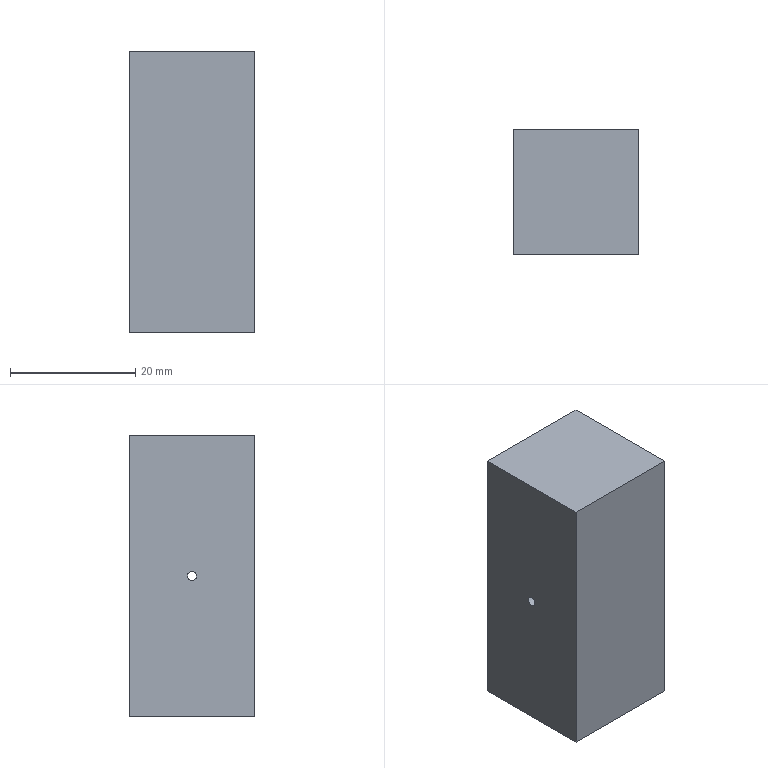Part | STEP file | SN10_016_001-02_BLOCO | 1 solid | 8 faces | box 20 x 20 x 45 mm | volume 16964 mm3 | plane 6 | cylinder 1 | cone 1 | commonest cylinder face diameters 8.376 x1
STEP:
#1=CARTESIAN_POINT('',(0.,0.,0.));
#2=DIRECTION('',(0.,0.,1.));
#3=DIRECTION('',(1.,0.,0.));
#4=AXIS2_PLACEMENT_3D('',#1,#2,#3);
#5=CARTESIAN_POINT('',(5341.,-1241.325,70.492));
#6=VERTEX_POINT('',#5);
#7=CARTESIAN_POINT('',(5341.,-1245.,72.5));
#8=DIRECTION('',(-1.,0.,0.));
#9=DIRECTION('',(0.,1.,0.));
#10=AXIS2_PLACEMENT_3D('',#7,#8,#9);
#11=CIRCLE('',#10,4.188);
#12=CARTESIAN_POINT('',(5340.9,-1245.,72.5));
#13=DIRECTION('',(-1.,0.,0.));
#14=DIRECTION('',(0.,0.8776,-0.4794));
#15=AXIS2_PLACEMENT_3D('',#12,#13,#14);
#16=CYLINDRICAL_SURFACE('',#15,4.188);
#17=CARTESIAN_POINT('',(-0.5,-0.1));
#18=DIRECTION('',(1.,0.));
#19=VECTOR('',#18,1.);
#20=LINE('',#17,#19);
#21=(GEOMETRIC_REPRESENTATION_CONTEXT(2)PARAMETRIC_REPRESENTATION_CONTEXT()REPRESENTATION_CONTEXT('',''));
#22=DEFINITIONAL_REPRESENTATION('',(#20),#21);
#23=PCURVE('',#16,#22);
#24=CARTESIAN_POINT('',(5341.,0.,0.));
#25=DIRECTION('',(1.,0.,0.));
#26=DIRECTION('',(0.,0.,-1.));
#27=AXIS2_PLACEMENT_3D('',#24,#25,#26);
#28=PLANE('',#27);
#29=CARTESIAN_POINT('',(-72.5,-1240.812));
#30=CARTESIAN_POINT('',(-65.246,-1240.812));
#31=CARTESIAN_POINT('',(-68.873,-1247.094));
#32=CARTESIAN_POINT('',(-72.5,-1253.376));
#33=CARTESIAN_POINT('',(-76.127,-1247.094));
#34=CARTESIAN_POINT('',(-79.754,-1240.812));
#35=CARTESIAN_POINT('',(-72.5,-1240.812));
#36=(BOUNDED_CURVE()B_SPLINE_CURVE(2,(#29,#30,#31,#32,#33,#34,#35),.UNSPECIFIED.,.T.,.F.)B_SPLINE_CURVE_WITH_KNOTS((1,2,2,2,2,1),(-2.094,0.,2.094,4.189,6.283,8.378),.UNSPECIFIED.)CURVE()GEOMETRIC_REPRESENTATION_ITEM()RATIONAL_B_SPLINE_CURVE((1.,0.5,1.,0.5,1.,0.5,1.))REPRESENTATION_ITEM(''));
#37=(GEOMETRIC_REPRESENTATION_CONTEXT(2)PARAMETRIC_REPRESENTATION_CONTEXT()REPRESENTATION_CONTEXT('',''));
#38=DEFINITIONAL_REPRESENTATION('',(#36),#37);
#39=PCURVE('',#28,#38);
#40=SURFACE_CURVE('',#11,(#23,#39),.PCURVE_S1.);
#41=EDGE_CURVE('',#6,#6,#40,.T.);
#42=ORIENTED_EDGE('',*,*,#41,.T.);
#43=CARTESIAN_POINT('',(5323.,-1241.325,70.492));
#44=VERTEX_POINT('',#43);
#45=CARTESIAN_POINT('',(5341.,-1241.325,70.492));
#46=CARTESIAN_POINT('',(5323.,-1241.325,70.492));
#47=B_SPLINE_CURVE_WITH_KNOTS('',1,(#45,#46),.UNSPECIFIED.,.F.,.F.,(2,2),(-0.1,17.9),.PIECEWISE_BEZIER_KNOTS.);
#48=CARTESIAN_POINT('',(6.283,0.));
#49=DIRECTION('',(0.,1.));
#50=VECTOR('',#49,1.);
#51=LINE('',#48,#50);
#52=(GEOMETRIC_REPRESENTATION_CONTEXT(2)PARAMETRIC_REPRESENTATION_CONTEXT()REPRESENTATION_CONTEXT('',''));
#53=DEFINITIONAL_REPRESENTATION('',(#51),#52);
#54=PCURVE('',#16,#53);
#55=CARTESIAN_POINT('',(0.,0.));
#56=DIRECTION('',(0.,1.));
#57=VECTOR('',#56,1.);
#58=LINE('',#55,#57);
#59=(GEOMETRIC_REPRESENTATION_CONTEXT(2)PARAMETRIC_REPRESENTATION_CONTEXT()REPRESENTATION_CONTEXT('',''));
#60=DEFINITIONAL_REPRESENTATION('',(#58),#59);
#61=PCURVE('',#16,#60);
#62=SEAM_CURVE('',#47,(#54,#61),.PCURVE_S1.);
#63=EDGE_CURVE('',#6,#44,#62,.T.);
#64=ORIENTED_EDGE('',*,*,#63,.T.);
#65=CARTESIAN_POINT('',(5323.,-1245.,72.5));
#66=DIRECTION('',(-1.,0.,0.));
#67=DIRECTION('',(0.,1.,0.));
#68=AXIS2_PLACEMENT_3D('',#65,#66,#67);
#69=CIRCLE('',#68,4.188);
#70=CARTESIAN_POINT('',(-0.5,17.9));
#71=DIRECTION('',(1.,0.));
#72=VECTOR('',#71,1.);
#73=LINE('',#70,#72);
#74=(GEOMETRIC_REPRESENTATION_CONTEXT(2)PARAMETRIC_REPRESENTATION_CONTEXT()REPRESENTATION_CONTEXT('',''));
#75=DEFINITIONAL_REPRESENTATION('',(#73),#74);
#76=PCURVE('',#16,#75);
#77=CARTESIAN_POINT('',(5321.159,-1245.,72.5));
#78=DIRECTION('',(1.,0.,0.));
#79=DIRECTION('',(0.,0.8776,-0.4794));
#80=AXIS2_PLACEMENT_3D('',#77,#78,#79);
#81=CONICAL_SURFACE('',#80,1.,1.047);
#82=CARTESIAN_POINT('',(6.783,1.841));
#83=DIRECTION('',(-1.,0.));
#84=VECTOR('',#83,1.);
#85=LINE('',#82,#84);
#86=(GEOMETRIC_REPRESENTATION_CONTEXT(2)PARAMETRIC_REPRESENTATION_CONTEXT()REPRESENTATION_CONTEXT('',''));
#87=DEFINITIONAL_REPRESENTATION('',(#85),#86);
#88=PCURVE('',#81,#87);
#89=SURFACE_CURVE('',#69,(#76,#88),.PCURVE_S1.);
#90=EDGE_CURVE('',#44,#44,#89,.T.);
#91=ORIENTED_EDGE('',*,*,#90,.F.);
#92=ORIENTED_EDGE('',*,*,#63,.F.);
#93=EDGE_LOOP('',(#42,#64,#91,#92));
#94=FACE_BOUND('',#93,.F.);
#95=ADVANCED_FACE('',(#94),#16,.F.);
#96=CARTESIAN_POINT('',(5321.,-1245.635,72.847));
#97=VERTEX_POINT('',#96);
#98=CARTESIAN_POINT('',(5321.,-1244.365,72.153));
#99=VERTEX_POINT('',#98);
#100=CARTESIAN_POINT('',(5321.,-1245.,72.5));
#101=DIRECTION('',(1.,0.,0.));
#102=DIRECTION('',(0.,1.,0.));
#103=AXIS2_PLACEMENT_3D('',#100,#101,#102);
#104=CIRCLE('',#103,0.7239);
#105=CARTESIAN_POINT('',(0.5,-0.1594));
#106=DIRECTION('',(1.,0.));
#107=VECTOR('',#106,1.);
#108=LINE('',#105,#107);
#109=(GEOMETRIC_REPRESENTATION_CONTEXT(2)PARAMETRIC_REPRESENTATION_CONTEXT()REPRESENTATION_CONTEXT('',''));
#110=DEFINITIONAL_REPRESENTATION('',(#108),#109);
#111=PCURVE('',#81,#110);
#112=CARTESIAN_POINT('',(5321.,0.,0.));
#113=DIRECTION('',(1.,0.,0.));
#114=DIRECTION('',(0.,0.,-1.));
#115=AXIS2_PLACEMENT_3D('',#112,#113,#114);
#116=PLANE('',#115);
#117=CARTESIAN_POINT('',(-72.5,-1245.));
#118=DIRECTION('',(0.,1.));
#119=AXIS2_PLACEMENT_2D('',#117,#118);
#120=CIRCLE('',#119,0.7239);
#121=(GEOMETRIC_REPRESENTATION_CONTEXT(2)PARAMETRIC_REPRESENTATION_CONTEXT()REPRESENTATION_CONTEXT('',''));
#122=DEFINITIONAL_REPRESENTATION('',(#120),#121);
#123=PCURVE('',#116,#122);
#124=SURFACE_CURVE('',#104,(#111,#123),.PCURVE_S1.);
#125=EDGE_CURVE('',#97,#99,#124,.T.);
#126=ORIENTED_EDGE('',*,*,#125,.T.);
#127=CARTESIAN_POINT('',(5321.,-1244.365,72.153));
#128=CARTESIAN_POINT('',(5323.,-1241.325,70.492));
#129=B_SPLINE_CURVE_WITH_KNOTS('',1,(#127,#128),.UNSPECIFIED.,.F.,.F.,(2,2),(-0.3188,3.681),.PIECEWISE_BEZIER_KNOTS.);
#130=CARTESIAN_POINT('',(6.283,0.));
#131=DIRECTION('',(0.,1.));
#132=VECTOR('',#131,1.);
#133=LINE('',#130,#132);
#134=(GEOMETRIC_REPRESENTATION_CONTEXT(2)PARAMETRIC_REPRESENTATION_CONTEXT()REPRESENTATION_CONTEXT('',''));
#135=DEFINITIONAL_REPRESENTATION('',(#133),#134);
#136=PCURVE('',#81,#135);
#137=CARTESIAN_POINT('',(0.,0.));
#138=DIRECTION('',(0.,1.));
#139=VECTOR('',#138,1.);
#140=LINE('',#137,#139);
#141=(GEOMETRIC_REPRESENTATION_CONTEXT(2)PARAMETRIC_REPRESENTATION_CONTEXT()REPRESENTATION_CONTEXT('',''));
#142=DEFINITIONAL_REPRESENTATION('',(#140),#141);
#143=PCURVE('',#81,#142);
#144=SEAM_CURVE('',#129,(#136,#143),.PCURVE_S1.);
#145=EDGE_CURVE('',#99,#44,#144,.T.);
#146=ORIENTED_EDGE('',*,*,#145,.T.);
#147=ORIENTED_EDGE('',*,*,#90,.T.);
#148=ORIENTED_EDGE('',*,*,#145,.F.);
#149=CARTESIAN_POINT('',(5321.,-1245.,72.5));
#150=DIRECTION('',(1.,0.,0.));
#151=DIRECTION('',(0.,1.,0.));
#152=AXIS2_PLACEMENT_3D('',#149,#150,#151);
#153=CIRCLE('',#152,0.7239);
#154=CARTESIAN_POINT('',(-5.783,-0.1594));
#155=DIRECTION('',(1.,0.));
#156=VECTOR('',#155,1.);
#157=LINE('',#154,#156);
#158=(GEOMETRIC_REPRESENTATION_CONTEXT(2)PARAMETRIC_REPRESENTATION_CONTEXT()REPRESENTATION_CONTEXT('',''));
#159=DEFINITIONAL_REPRESENTATION('',(#157),#158);
#160=PCURVE('',#81,#159);
#161=CARTESIAN_POINT('',(-72.5,-1245.));
#162=DIRECTION('',(0.,1.));
#163=AXIS2_PLACEMENT_2D('',#161,#162);
#164=CIRCLE('',#163,0.7239);
#165=(GEOMETRIC_REPRESENTATION_CONTEXT(2)PARAMETRIC_REPRESENTATION_CONTEXT()REPRESENTATION_CONTEXT('',''));
#166=DEFINITIONAL_REPRESENTATION('',(#164),#165);
#167=PCURVE('',#116,#166);
#168=SURFACE_CURVE('',#153,(#160,#167),.PCURVE_S1.);
#169=EDGE_CURVE('',#99,#97,#168,.T.);
#170=ORIENTED_EDGE('',*,*,#169,.T.);
#171=EDGE_LOOP('',(#126,#146,#147,#148,#170));
#172=FACE_BOUND('',#171,.F.);
#173=ADVANCED_FACE('',(#172),#81,.F.);
#174=CARTESIAN_POINT('',(5341.,-1255.,95.));
#175=VERTEX_POINT('',#174);
#176=CARTESIAN_POINT('',(5341.,-1255.,50.));
#177=VERTEX_POINT('',#176);
#178=CARTESIAN_POINT('',(5341.,-1255.,95.));
#179=DIRECTION('',(0.,0.,-1.));
#180=VECTOR('',#179,1.);
#181=LINE('',#178,#180);
#182=CARTESIAN_POINT('',(-95.,-1255.));
#183=DIRECTION('',(1.,0.));
#184=VECTOR('',#183,1.);
#185=LINE('',#182,#184);
#186=(GEOMETRIC_REPRESENTATION_CONTEXT(2)PARAMETRIC_REPRESENTATION_CONTEXT()REPRESENTATION_CONTEXT('',''));
#187=DEFINITIONAL_REPRESENTATION('',(#185),#186);
#188=PCURVE('',#28,#187);
#189=CARTESIAN_POINT('',(5321.,-1255.,95.));
#190=DIRECTION('',(0.,-1.,0.));
#191=DIRECTION('',(0.,0.,-1.));
#192=AXIS2_PLACEMENT_3D('',#189,#190,#191);
#193=PLANE('',#192);
#194=CARTESIAN_POINT('',(0.,20.));
#195=DIRECTION('',(1.,0.));
#196=VECTOR('',#195,1.);
#197=LINE('',#194,#196);
#198=(GEOMETRIC_REPRESENTATION_CONTEXT(2)PARAMETRIC_REPRESENTATION_CONTEXT()REPRESENTATION_CONTEXT('',''));
#199=DEFINITIONAL_REPRESENTATION('',(#197),#198);
#200=PCURVE('',#193,#199);
#201=SURFACE_CURVE('',#181,(#188,#200),.PCURVE_S1.);
#202=EDGE_CURVE('',#175,#177,#201,.T.);
#203=ORIENTED_EDGE('',*,*,#202,.T.);
#204=CARTESIAN_POINT('',(5341.,-1235.,50.));
#205=VERTEX_POINT('',#204);
#206=CARTESIAN_POINT('',(5341.,-1235.,50.));
#207=DIRECTION('',(0.,-1.,0.));
#208=VECTOR('',#207,1.);
#209=LINE('',#206,#208);
#210=CARTESIAN_POINT('',(-50.,-1235.));
#211=DIRECTION('',(0.,-1.));
#212=VECTOR('',#211,1.);
#213=LINE('',#210,#212);
#214=(GEOMETRIC_REPRESENTATION_CONTEXT(2)PARAMETRIC_REPRESENTATION_CONTEXT()REPRESENTATION_CONTEXT('',''));
#215=DEFINITIONAL_REPRESENTATION('',(#213),#214);
#216=PCURVE('',#28,#215);
#217=CARTESIAN_POINT('',(5321.,-1235.,50.));
#218=DIRECTION('',(0.,0.,1.));
#219=DIRECTION('',(1.,0.,0.));
#220=AXIS2_PLACEMENT_3D('',#217,#218,#219);
#221=PLANE('',#220);
#222=CARTESIAN_POINT('',(20.,0.));
#223=DIRECTION('',(0.,-1.));
#224=VECTOR('',#223,1.);
#225=LINE('',#222,#224);
#226=(GEOMETRIC_REPRESENTATION_CONTEXT(2)PARAMETRIC_REPRESENTATION_CONTEXT()REPRESENTATION_CONTEXT('',''));
#227=DEFINITIONAL_REPRESENTATION('',(#225),#226);
#228=PCURVE('',#221,#227);
#229=SURFACE_CURVE('',#209,(#216,#228),.PCURVE_S1.);
#230=EDGE_CURVE('',#205,#177,#229,.T.);
#231=ORIENTED_EDGE('',*,*,#230,.F.);
#232=CARTESIAN_POINT('',(5341.,-1235.,95.));
#233=VERTEX_POINT('',#232);
#234=CARTESIAN_POINT('',(5341.,-1235.,50.));
#235=DIRECTION('',(0.,0.,1.));
#236=VECTOR('',#235,1.);
#237=LINE('',#234,#236);
#238=CARTESIAN_POINT('',(-50.,-1235.));
#239=DIRECTION('',(-1.,0.));
#240=VECTOR('',#239,1.);
#241=LINE('',#238,#240);
#242=(GEOMETRIC_REPRESENTATION_CONTEXT(2)PARAMETRIC_REPRESENTATION_CONTEXT()REPRESENTATION_CONTEXT('',''));
#243=DEFINITIONAL_REPRESENTATION('',(#241),#242);
#244=PCURVE('',#28,#243);
#245=CARTESIAN_POINT('',(5321.,-1235.,50.));
#246=DIRECTION('',(0.,1.,0.));
#247=DIRECTION('',(0.,0.,1.));
#248=AXIS2_PLACEMENT_3D('',#245,#246,#247);
#249=PLANE('',#248);
#250=CARTESIAN_POINT('',(0.,20.));
#251=DIRECTION('',(1.,0.));
#252=VECTOR('',#251,1.);
#253=LINE('',#250,#252);
#254=(GEOMETRIC_REPRESENTATION_CONTEXT(2)PARAMETRIC_REPRESENTATION_CONTEXT()REPRESENTATION_CONTEXT('',''));
#255=DEFINITIONAL_REPRESENTATION('',(#253),#254);
#256=PCURVE('',#249,#255);
#257=SURFACE_CURVE('',#237,(#244,#256),.PCURVE_S1.);
#258=EDGE_CURVE('',#205,#233,#257,.T.);
#259=ORIENTED_EDGE('',*,*,#258,.T.);
#260=CARTESIAN_POINT('',(5341.,-1255.,95.));
#261=DIRECTION('',(0.,1.,0.));
#262=VECTOR('',#261,1.);
#263=LINE('',#260,#262);
#264=CARTESIAN_POINT('',(-95.,-1255.));
#265=DIRECTION('',(0.,1.));
#266=VECTOR('',#265,1.);
#267=LINE('',#264,#266);
#268=(GEOMETRIC_REPRESENTATION_CONTEXT(2)PARAMETRIC_REPRESENTATION_CONTEXT()REPRESENTATION_CONTEXT('',''));
#269=DEFINITIONAL_REPRESENTATION('',(#267),#268);
#270=PCURVE('',#28,#269);
#271=CARTESIAN_POINT('',(5321.,-1255.,95.));
#272=DIRECTION('',(0.,0.,-1.));
#273=DIRECTION('',(-1.,0.,0.));
#274=AXIS2_PLACEMENT_3D('',#271,#272,#273);
#275=PLANE('',#274);
#276=CARTESIAN_POINT('',(-20.,0.));
#277=DIRECTION('',(0.,1.));
#278=VECTOR('',#277,1.);
#279=LINE('',#276,#278);
#280=(GEOMETRIC_REPRESENTATION_CONTEXT(2)PARAMETRIC_REPRESENTATION_CONTEXT()REPRESENTATION_CONTEXT('',''));
#281=DEFINITIONAL_REPRESENTATION('',(#279),#280);
#282=PCURVE('',#275,#281);
#283=SURFACE_CURVE('',#263,(#270,#282),.PCURVE_S1.);
#284=EDGE_CURVE('',#175,#233,#283,.T.);
#285=ORIENTED_EDGE('',*,*,#284,.F.);
#286=EDGE_LOOP('',(#203,#231,#259,#285));
#287=FACE_BOUND('',#286,.T.);
#288=ORIENTED_EDGE('',*,*,#41,.T.);
#289=EDGE_LOOP('',(#288));
#290=FACE_BOUND('',#289,.T.);
#291=ADVANCED_FACE('',(#287,#290),#28,.T.);
#292=CARTESIAN_POINT('',(5321.,-1255.,95.));
#293=VERTEX_POINT('',#292);
#294=CARTESIAN_POINT('',(5321.,-1255.,95.));
#295=DIRECTION('',(1.,0.,0.));
#296=VECTOR('',#295,1.);
#297=LINE('',#294,#296);
#298=CARTESIAN_POINT('',(0.,0.));
#299=DIRECTION('',(0.,1.));
#300=VECTOR('',#299,1.);
#301=LINE('',#298,#300);
#302=(GEOMETRIC_REPRESENTATION_CONTEXT(2)PARAMETRIC_REPRESENTATION_CONTEXT()REPRESENTATION_CONTEXT('',''));
#303=DEFINITIONAL_REPRESENTATION('',(#301),#302);
#304=PCURVE('',#193,#303);
#305=CARTESIAN_POINT('',(0.,0.));
#306=DIRECTION('',(-1.,0.));
#307=VECTOR('',#306,1.);
#308=LINE('',#305,#307);
#309=(GEOMETRIC_REPRESENTATION_CONTEXT(2)PARAMETRIC_REPRESENTATION_CONTEXT()REPRESENTATION_CONTEXT('',''));
#310=DEFINITIONAL_REPRESENTATION('',(#308),#309);
#311=PCURVE('',#275,#310);
#312=SURFACE_CURVE('',#297,(#304,#311),.PCURVE_S1.);
#313=EDGE_CURVE('',#293,#175,#312,.T.);
#314=ORIENTED_EDGE('',*,*,#313,.F.);
#315=CARTESIAN_POINT('',(5321.,-1255.,50.));
#316=VERTEX_POINT('',#315);
#317=CARTESIAN_POINT('',(5321.,-1255.,95.));
#318=DIRECTION('',(0.,0.,-1.));
#319=VECTOR('',#318,1.);
#320=LINE('',#317,#319);
#321=CARTESIAN_POINT('',(0.,0.));
#322=DIRECTION('',(1.,0.));
#323=VECTOR('',#322,1.);
#324=LINE('',#321,#323);
#325=(GEOMETRIC_REPRESENTATION_CONTEXT(2)PARAMETRIC_REPRESENTATION_CONTEXT()REPRESENTATION_CONTEXT('',''));
#326=DEFINITIONAL_REPRESENTATION('',(#324),#325);
#327=PCURVE('',#193,#326);
#328=CARTESIAN_POINT('',(-95.,-1255.));
#329=DIRECTION('',(1.,0.));
#330=VECTOR('',#329,1.);
#331=LINE('',#328,#330);
#332=(GEOMETRIC_REPRESENTATION_CONTEXT(2)PARAMETRIC_REPRESENTATION_CONTEXT()REPRESENTATION_CONTEXT('',''));
#333=DEFINITIONAL_REPRESENTATION('',(#331),#332);
#334=PCURVE('',#116,#333);
#335=SURFACE_CURVE('',#320,(#327,#334),.PCURVE_S1.);
#336=EDGE_CURVE('',#293,#316,#335,.T.);
#337=ORIENTED_EDGE('',*,*,#336,.T.);
#338=CARTESIAN_POINT('',(5321.,-1255.,50.));
#339=DIRECTION('',(1.,0.,0.));
#340=VECTOR('',#339,1.);
#341=LINE('',#338,#340);
#342=CARTESIAN_POINT('',(45.,0.));
#343=DIRECTION('',(0.,1.));
#344=VECTOR('',#343,1.);
#345=LINE('',#342,#344);
#346=(GEOMETRIC_REPRESENTATION_CONTEXT(2)PARAMETRIC_REPRESENTATION_CONTEXT()REPRESENTATION_CONTEXT('',''));
#347=DEFINITIONAL_REPRESENTATION('',(#345),#346);
#348=PCURVE('',#193,#347);
#349=CARTESIAN_POINT('',(0.,-20.));
#350=DIRECTION('',(1.,0.));
#351=VECTOR('',#350,1.);
#352=LINE('',#349,#351);
#353=(GEOMETRIC_REPRESENTATION_CONTEXT(2)PARAMETRIC_REPRESENTATION_CONTEXT()REPRESENTATION_CONTEXT('',''));
#354=DEFINITIONAL_REPRESENTATION('',(#352),#353);
#355=PCURVE('',#221,#354);
#356=SURFACE_CURVE('',#341,(#348,#355),.PCURVE_S1.);
#357=EDGE_CURVE('',#316,#177,#356,.T.);
#358=ORIENTED_EDGE('',*,*,#357,.T.);
#359=ORIENTED_EDGE('',*,*,#202,.F.);
#360=EDGE_LOOP('',(#314,#337,#358,#359));
#361=FACE_BOUND('',#360,.T.);
#362=ADVANCED_FACE('',(#361),#193,.T.);
#363=ORIENTED_EDGE('',*,*,#357,.F.);
#364=CARTESIAN_POINT('',(5321.,-1235.,50.));
#365=VERTEX_POINT('',#364);
#366=CARTESIAN_POINT('',(5321.,-1235.,50.));
#367=DIRECTION('',(0.,-1.,0.));
#368=VECTOR('',#367,1.);
#369=LINE('',#366,#368);
#370=CARTESIAN_POINT('',(0.,0.));
#371=DIRECTION('',(0.,-1.));
#372=VECTOR('',#371,1.);
#373=LINE('',#370,#372);
#374=(GEOMETRIC_REPRESENTATION_CONTEXT(2)PARAMETRIC_REPRESENTATION_CONTEXT()REPRESENTATION_CONTEXT('',''));
#375=DEFINITIONAL_REPRESENTATION('',(#373),#374);
#376=PCURVE('',#221,#375);
#377=CARTESIAN_POINT('',(-50.,-1235.));
#378=DIRECTION('',(0.,-1.));
#379=VECTOR('',#378,1.);
#380=LINE('',#377,#379);
#381=(GEOMETRIC_REPRESENTATION_CONTEXT(2)PARAMETRIC_REPRESENTATION_CONTEXT()REPRESENTATION_CONTEXT('',''));
#382=DEFINITIONAL_REPRESENTATION('',(#380),#381);
#383=PCURVE('',#116,#382);
#384=SURFACE_CURVE('',#369,(#376,#383),.PCURVE_S1.);
#385=EDGE_CURVE('',#365,#316,#384,.T.);
#386=ORIENTED_EDGE('',*,*,#385,.F.);
#387=CARTESIAN_POINT('',(5321.,-1235.,50.));
#388=DIRECTION('',(1.,0.,0.));
#389=VECTOR('',#388,1.);
#390=LINE('',#387,#389);
#391=CARTESIAN_POINT('',(0.,0.));
#392=DIRECTION('',(1.,0.));
#393=VECTOR('',#392,1.);
#394=LINE('',#391,#393);
#395=(GEOMETRIC_REPRESENTATION_CONTEXT(2)PARAMETRIC_REPRESENTATION_CONTEXT()REPRESENTATION_CONTEXT('',''));
#396=DEFINITIONAL_REPRESENTATION('',(#394),#395);
#397=PCURVE('',#221,#396);
#398=CARTESIAN_POINT('',(0.,0.));
#399=DIRECTION('',(0.,1.));
#400=VECTOR('',#399,1.);
#401=LINE('',#398,#400);
#402=(GEOMETRIC_REPRESENTATION_CONTEXT(2)PARAMETRIC_REPRESENTATION_CONTEXT()REPRESENTATION_CONTEXT('',''));
#403=DEFINITIONAL_REPRESENTATION('',(#401),#402);
#404=PCURVE('',#249,#403);
#405=SURFACE_CURVE('',#390,(#397,#404),.PCURVE_S1.);
#406=EDGE_CURVE('',#365,#205,#405,.T.);
#407=ORIENTED_EDGE('',*,*,#406,.T.);
#408=ORIENTED_EDGE('',*,*,#230,.T.);
#409=EDGE_LOOP('',(#363,#386,#407,#408));
#410=FACE_BOUND('',#409,.T.);
#411=ADVANCED_FACE('',(#410),#221,.F.);
#412=ORIENTED_EDGE('',*,*,#406,.F.);
#413=CARTESIAN_POINT('',(5321.,-1235.,95.));
#414=VERTEX_POINT('',#413);
#415=CARTESIAN_POINT('',(5321.,-1235.,50.));
#416=DIRECTION('',(0.,0.,1.));
#417=VECTOR('',#416,1.);
#418=LINE('',#415,#417);
#419=CARTESIAN_POINT('',(0.,0.));
#420=DIRECTION('',(1.,0.));
#421=VECTOR('',#420,1.);
#422=LINE('',#419,#421);
#423=(GEOMETRIC_REPRESENTATION_CONTEXT(2)PARAMETRIC_REPRESENTATION_CONTEXT()REPRESENTATION_CONTEXT('',''));
#424=DEFINITIONAL_REPRESENTATION('',(#422),#423);
#425=PCURVE('',#249,#424);
#426=CARTESIAN_POINT('',(-50.,-1235.));
#427=DIRECTION('',(-1.,0.));
#428=VECTOR('',#427,1.);
#429=LINE('',#426,#428);
#430=(GEOMETRIC_REPRESENTATION_CONTEXT(2)PARAMETRIC_REPRESENTATION_CONTEXT()REPRESENTATION_CONTEXT('',''));
#431=DEFINITIONAL_REPRESENTATION('',(#429),#430);
#432=PCURVE('',#116,#431);
#433=SURFACE_CURVE('',#418,(#425,#432),.PCURVE_S1.);
#434=EDGE_CURVE('',#365,#414,#433,.T.);
#435=ORIENTED_EDGE('',*,*,#434,.T.);
#436=CARTESIAN_POINT('',(5321.,-1235.,95.));
#437=DIRECTION('',(1.,0.,0.));
#438=VECTOR('',#437,1.);
#439=LINE('',#436,#438);
#440=CARTESIAN_POINT('',(45.,0.));
#441=DIRECTION('',(0.,1.));
#442=VECTOR('',#441,1.);
#443=LINE('',#440,#442);
#444=(GEOMETRIC_REPRESENTATION_CONTEXT(2)PARAMETRIC_REPRESENTATION_CONTEXT()REPRESENTATION_CONTEXT('',''));
#445=DEFINITIONAL_REPRESENTATION('',(#443),#444);
#446=PCURVE('',#249,#445);
#447=CARTESIAN_POINT('',(0.,20.));
#448=DIRECTION('',(-1.,0.));
#449=VECTOR('',#448,1.);
#450=LINE('',#447,#449);
#451=(GEOMETRIC_REPRESENTATION_CONTEXT(2)PARAMETRIC_REPRESENTATION_CONTEXT()REPRESENTATION_CONTEXT('',''));
#452=DEFINITIONAL_REPRESENTATION('',(#450),#451);
#453=PCURVE('',#275,#452);
#454=SURFACE_CURVE('',#439,(#446,#453),.PCURVE_S1.);
#455=EDGE_CURVE('',#414,#233,#454,.T.);
#456=ORIENTED_EDGE('',*,*,#455,.T.);
#457=ORIENTED_EDGE('',*,*,#258,.F.);
#458=EDGE_LOOP('',(#412,#435,#456,#457));
#459=FACE_BOUND('',#458,.T.);
#460=ADVANCED_FACE('',(#459),#249,.T.);
#461=ORIENTED_EDGE('',*,*,#455,.F.);
#462=CARTESIAN_POINT('',(5321.,-1255.,95.));
#463=DIRECTION('',(0.,1.,0.));
#464=VECTOR('',#463,1.);
#465=LINE('',#462,#464);
#466=CARTESIAN_POINT('',(0.,0.));
#467=DIRECTION('',(0.,1.));
#468=VECTOR('',#467,1.);
#469=LINE('',#466,#468);
#470=(GEOMETRIC_REPRESENTATION_CONTEXT(2)PARAMETRIC_REPRESENTATION_CONTEXT()REPRESENTATION_CONTEXT('',''));
#471=DEFINITIONAL_REPRESENTATION('',(#469),#470);
#472=PCURVE('',#275,#471);
#473=CARTESIAN_POINT('',(-95.,-1255.));
#474=DIRECTION('',(0.,1.));
#475=VECTOR('',#474,1.);
#476=LINE('',#473,#475);
#477=(GEOMETRIC_REPRESENTATION_CONTEXT(2)PARAMETRIC_REPRESENTATION_CONTEXT()REPRESENTATION_CONTEXT('',''));
#478=DEFINITIONAL_REPRESENTATION('',(#476),#477);
#479=PCURVE('',#116,#478);
#480=SURFACE_CURVE('',#465,(#472,#479),.PCURVE_S1.);
#481=EDGE_CURVE('',#293,#414,#480,.T.);
#482=ORIENTED_EDGE('',*,*,#481,.F.);
#483=ORIENTED_EDGE('',*,*,#313,.T.);
#484=ORIENTED_EDGE('',*,*,#284,.T.);
#485=EDGE_LOOP('',(#461,#482,#483,#484));
#486=FACE_BOUND('',#485,.T.);
#487=ADVANCED_FACE('',(#486),#275,.F.);
#488=ORIENTED_EDGE('',*,*,#481,.T.);
#489=ORIENTED_EDGE('',*,*,#434,.F.);
#490=ORIENTED_EDGE('',*,*,#385,.T.);
#491=ORIENTED_EDGE('',*,*,#336,.F.);
#492=EDGE_LOOP('',(#488,#489,#490,#491));
#493=FACE_BOUND('',#492,.T.);
#494=ORIENTED_EDGE('',*,*,#125,.T.);
#495=ORIENTED_EDGE('',*,*,#169,.T.);
#496=EDGE_LOOP('',(#494,#495));
#497=FACE_BOUND('',#496,.T.);
#498=ADVANCED_FACE('',(#493,#497),#116,.F.);
#499=CLOSED_SHELL('',(#95,#173,#291,#362,#411,#460,#487,#498));
#500=MANIFOLD_SOLID_BREP('',#499);
#501=(LENGTH_UNIT()NAMED_UNIT(*)SI_UNIT(.MILLI.,.METRE.));
#502=UNCERTAINTY_MEASURE_WITH_UNIT(LENGTH_MEASURE(0.000002),#501,'','');
#503=(NAMED_UNIT(*)PLANE_ANGLE_UNIT()SI_UNIT($,.RADIAN.));
#504=(NAMED_UNIT(*)SI_UNIT($,.STERADIAN.)SOLID_ANGLE_UNIT());
#505=(GEOMETRIC_REPRESENTATION_CONTEXT(3)GLOBAL_UNCERTAINTY_ASSIGNED_CONTEXT((#502))GLOBAL_UNIT_ASSIGNED_CONTEXT((#501,#503,#504))REPRESENTATION_CONTEXT('',''));
#506=ADVANCED_BREP_SHAPE_REPRESENTATION('',(#4,#500),#505);